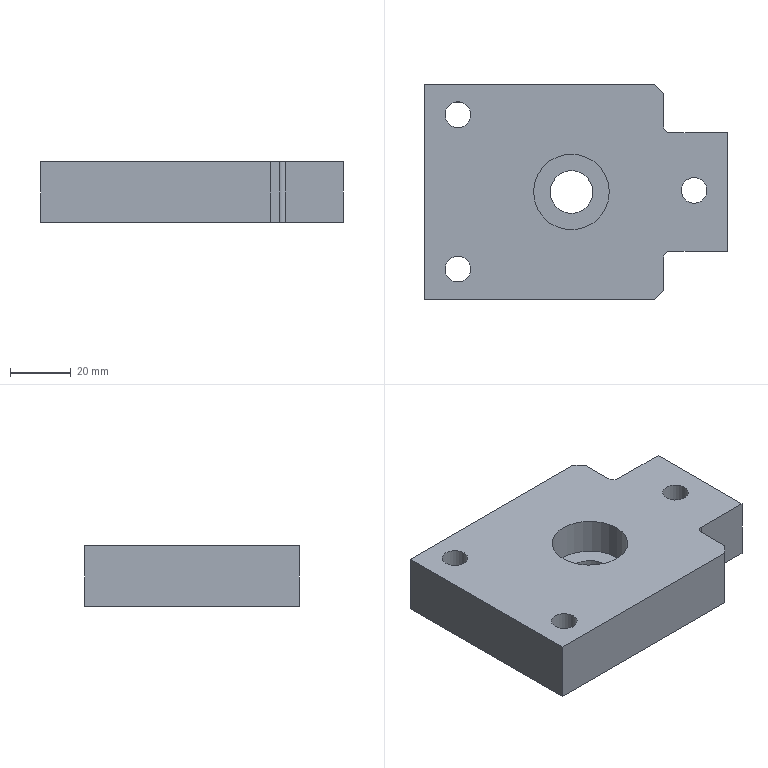Part | NX | features solid 2 | 1 solid | 26 faces | box 100 x 71 x 20 mm | volume 115003 mm3 | plane 16 | cylinder 10 | commonest cylinder face diameters 8.5 x3 14 x3 4 x2 14.1 x1 25 x1
STEP:
#1=CARTESIAN_POINT('',(232.75,0.5,10.));
#2=VERTEX_POINT('',#1);
#3=CARTESIAN_POINT('',(228.5,0.5,10.));
#4=DIRECTION('',(0.,0.,1.));
#5=DIRECTION('',(1.,0.,0.));
#6=AXIS2_PLACEMENT_3D('',#3,#4,#5);
#7=CIRCLE('',#6,4.25);
#8=EDGE_CURVE('',#2,#2,#7,.F.);
#9=ORIENTED_EDGE('',*,*,#8,.T.);
#10=EDGE_LOOP('',(#9));
#11=FACE_BOUND('',#10,.T.);
#12=CARTESIAN_POINT('',(232.75,0.5,20.));
#13=VERTEX_POINT('',#12);
#14=CARTESIAN_POINT('',(228.5,0.5,20.));
#15=DIRECTION('',(0.,0.,1.));
#16=DIRECTION('',(1.,0.,0.));
#17=AXIS2_PLACEMENT_3D('',#14,#15,#16);
#18=CIRCLE('',#17,4.25);
#19=EDGE_CURVE('',#13,#13,#18,.T.);
#20=ORIENTED_EDGE('',*,*,#19,.T.);
#21=EDGE_LOOP('',(#20));
#22=FACE_BOUND('',#21,.T.);
#23=CARTESIAN_POINT('',(228.5,0.5,40.));
#24=DIRECTION('',(0.,0.,1.));
#25=DIRECTION('',(1.,0.,0.));
#26=AXIS2_PLACEMENT_3D('',#23,#24,#25);
#27=CYLINDRICAL_SURFACE('',#26,4.25);
#28=ADVANCED_FACE('',(#11,#22),#27,.F.);
#29=ORIENTED_EDGE('',*,*,#8,.F.);
#30=EDGE_LOOP('',(#29));
#31=FACE_BOUND('',#30,.T.);
#32=CARTESIAN_POINT('',(235.5,0.5,10.));
#33=VERTEX_POINT('',#32);
#34=CARTESIAN_POINT('',(228.5,0.5,10.));
#35=DIRECTION('',(0.,0.,1.));
#36=DIRECTION('',(1.,0.,0.));
#37=AXIS2_PLACEMENT_3D('',#34,#35,#36);
#38=CIRCLE('',#37,7.);
#39=EDGE_CURVE('',#33,#33,#38,.F.);
#40=ORIENTED_EDGE('',*,*,#39,.T.);
#41=EDGE_LOOP('',(#40));
#42=FACE_BOUND('',#41,.T.);
#43=CARTESIAN_POINT('',(231.693,-4.466,10.));
#44=DIRECTION('',(0.,0.,1.));
#45=DIRECTION('',(1.,0.,0.));
#46=AXIS2_PLACEMENT_3D('',#43,#44,#45);
#47=PLANE('',#46);
#48=ADVANCED_FACE('',(#31,#42),#47,.F.);
#49=ORIENTED_EDGE('',*,*,#39,.F.);
#50=EDGE_LOOP('',(#49));
#51=FACE_BOUND('',#50,.T.);
#52=CARTESIAN_POINT('',(235.5,0.5,0.00000121));
#53=VERTEX_POINT('',#52);
#54=CARTESIAN_POINT('',(228.5,0.5,0.00000121));
#55=DIRECTION('',(0.,0.,1.));
#56=DIRECTION('',(1.,0.,0.));
#57=AXIS2_PLACEMENT_3D('',#54,#55,#56);
#58=CIRCLE('',#57,7.);
#59=EDGE_CURVE('',#53,#53,#58,.F.);
#60=ORIENTED_EDGE('',*,*,#59,.T.);
#61=EDGE_LOOP('',(#60));
#62=FACE_BOUND('',#61,.T.);
#63=CARTESIAN_POINT('',(228.5,0.5,0.00000121));
#64=DIRECTION('',(0.,0.,1.));
#65=DIRECTION('',(1.,0.,0.));
#66=AXIS2_PLACEMENT_3D('',#63,#64,#65);
#67=CYLINDRICAL_SURFACE('',#66,7.);
#68=ADVANCED_FACE('',(#51,#62),#67,.F.);
#69=CARTESIAN_POINT('',(154.75,-25.5,10.));
#70=VERTEX_POINT('',#69);
#71=CARTESIAN_POINT('',(150.5,-25.5,10.));
#72=DIRECTION('',(0.,0.,1.));
#73=DIRECTION('',(1.,0.,0.));
#74=AXIS2_PLACEMENT_3D('',#71,#72,#73);
#75=CIRCLE('',#74,4.25);
#76=EDGE_CURVE('',#70,#70,#75,.F.);
#77=ORIENTED_EDGE('',*,*,#76,.F.);
#78=EDGE_LOOP('',(#77));
#79=FACE_BOUND('',#78,.T.);
#80=CARTESIAN_POINT('',(157.5,-25.5,10.));
#81=VERTEX_POINT('',#80);
#82=CARTESIAN_POINT('',(150.5,-25.5,10.));
#83=DIRECTION('',(0.,0.,1.));
#84=DIRECTION('',(1.,0.,0.));
#85=AXIS2_PLACEMENT_3D('',#82,#83,#84);
#86=CIRCLE('',#85,7.);
#87=EDGE_CURVE('',#81,#81,#86,.F.);
#88=ORIENTED_EDGE('',*,*,#87,.T.);
#89=EDGE_LOOP('',(#88));
#90=FACE_BOUND('',#89,.T.);
#91=CARTESIAN_POINT('',(151.774,-24.174,10.));
#92=DIRECTION('',(0.,0.,1.));
#93=DIRECTION('',(1.,0.,0.));
#94=AXIS2_PLACEMENT_3D('',#91,#92,#93);
#95=PLANE('',#94);
#96=ADVANCED_FACE('',(#79,#90),#95,.F.);
#97=CARTESIAN_POINT('',(154.75,25.5,10.));
#98=VERTEX_POINT('',#97);
#99=CARTESIAN_POINT('',(150.5,25.5,10.));
#100=DIRECTION('',(0.,0.,-1.));
#101=DIRECTION('',(1.,0.,0.));
#102=AXIS2_PLACEMENT_3D('',#99,#100,#101);
#103=CIRCLE('',#102,4.25);
#104=EDGE_CURVE('',#98,#98,#103,.T.);
#105=ORIENTED_EDGE('',*,*,#104,.F.);
#106=EDGE_LOOP('',(#105));
#107=FACE_BOUND('',#106,.T.);
#108=CARTESIAN_POINT('',(157.5,25.5,10.));
#109=VERTEX_POINT('',#108);
#110=CARTESIAN_POINT('',(150.5,25.5,10.));
#111=DIRECTION('',(0.,0.,-1.));
#112=DIRECTION('',(1.,0.,0.));
#113=AXIS2_PLACEMENT_3D('',#110,#111,#112);
#114=CIRCLE('',#113,7.);
#115=EDGE_CURVE('',#109,#109,#114,.T.);
#116=ORIENTED_EDGE('',*,*,#115,.T.);
#117=EDGE_LOOP('',(#116));
#118=FACE_BOUND('',#117,.T.);
#119=CARTESIAN_POINT('',(151.774,24.174,10.));
#120=DIRECTION('',(0.,0.,1.));
#121=DIRECTION('',(1.,0.,0.));
#122=AXIS2_PLACEMENT_3D('',#119,#120,#121);
#123=PLANE('',#122);
#124=ADVANCED_FACE('',(#107,#118),#123,.F.);
#125=CARTESIAN_POINT('',(139.5,35.5,0.00000121));
#126=VERTEX_POINT('',#125);
#127=CARTESIAN_POINT('',(139.5,35.5,20.));
#128=VERTEX_POINT('',#127);
#129=CARTESIAN_POINT('',(139.5,35.5,70.));
#130=DIRECTION('',(0.,0.,1.));
#131=VECTOR('',#130,1000.);
#132=LINE('',#129,#131);
#133=EDGE_CURVE('',#126,#128,#132,.T.);
#134=ORIENTED_EDGE('',*,*,#133,.F.);
#135=CARTESIAN_POINT('',(139.5,-35.5,0.00000121));
#136=VERTEX_POINT('',#135);
#137=CARTESIAN_POINT('',(139.5,0.,0.00000121));
#138=DIRECTION('',(0.,1.,0.));
#139=VECTOR('',#138,1000.);
#140=LINE('',#137,#139);
#141=EDGE_CURVE('',#126,#136,#140,.F.);
#142=ORIENTED_EDGE('',*,*,#141,.T.);
#143=CARTESIAN_POINT('',(139.5,-35.5,20.));
#144=VERTEX_POINT('',#143);
#145=CARTESIAN_POINT('',(139.5,-35.5,70.));
#146=DIRECTION('',(0.,0.,-1.));
#147=VECTOR('',#146,1000.);
#148=LINE('',#145,#147);
#149=EDGE_CURVE('',#144,#136,#148,.T.);
#150=ORIENTED_EDGE('',*,*,#149,.F.);
#151=CARTESIAN_POINT('',(139.5,0.,20.));
#152=DIRECTION('',(0.,-1.,0.));
#153=VECTOR('',#152,1000.);
#154=LINE('',#151,#153);
#155=EDGE_CURVE('',#128,#144,#154,.T.);
#156=ORIENTED_EDGE('',*,*,#155,.F.);
#157=EDGE_LOOP('',(#134,#142,#150,#156));
#158=FACE_BOUND('',#157,.T.);
#159=CARTESIAN_POINT('',(139.5,0.,35.));
#160=DIRECTION('',(1.,0.,0.));
#161=DIRECTION('',(0.,-1.,0.));
#162=AXIS2_PLACEMENT_3D('',#159,#160,#161);
#163=PLANE('',#162);
#164=ADVANCED_FACE('',(#158),#163,.F.);
#165=ORIENTED_EDGE('',*,*,#149,.T.);
#166=CARTESIAN_POINT('',(215.5,-35.5,0.00000121));
#167=VERTEX_POINT('',#166);
#168=CARTESIAN_POINT('',(157.5,-35.5,0.00000121));
#169=DIRECTION('',(-1.,0.,0.));
#170=VECTOR('',#169,1000.);
#171=LINE('',#168,#170);
#172=EDGE_CURVE('',#136,#167,#171,.F.);
#173=ORIENTED_EDGE('',*,*,#172,.T.);
#174=CARTESIAN_POINT('',(215.5,-35.5,20.));
#175=VERTEX_POINT('',#174);
#176=CARTESIAN_POINT('',(215.5,-35.5,70.));
#177=DIRECTION('',(0.,0.,1.));
#178=VECTOR('',#177,1000.);
#179=LINE('',#176,#178);
#180=EDGE_CURVE('',#167,#175,#179,.T.);
#181=ORIENTED_EDGE('',*,*,#180,.T.);
#182=CARTESIAN_POINT('',(157.5,-35.5,20.));
#183=DIRECTION('',(1.,0.,0.));
#184=VECTOR('',#183,1000.);
#185=LINE('',#182,#184);
#186=EDGE_CURVE('',#144,#175,#185,.T.);
#187=ORIENTED_EDGE('',*,*,#186,.F.);
#188=EDGE_LOOP('',(#165,#173,#181,#187));
#189=FACE_BOUND('',#188,.T.);
#190=CARTESIAN_POINT('',(157.5,-35.5,70.));
#191=DIRECTION('',(0.,1.,0.));
#192=DIRECTION('',(-1.,0.,0.));
#193=AXIS2_PLACEMENT_3D('',#190,#191,#192);
#194=PLANE('',#193);
#195=ADVANCED_FACE('',(#189),#194,.F.);
#196=ORIENTED_EDGE('',*,*,#180,.F.);
#197=CARTESIAN_POINT('',(218.5,-32.5,0.00000121));
#198=VERTEX_POINT('',#197);
#199=CARTESIAN_POINT('',(219.5,-31.5,0.00000121));
#200=DIRECTION('',(0.7071,0.7071,0.));
#201=VECTOR('',#200,1000.);
#202=LINE('',#199,#201);
#203=EDGE_CURVE('',#198,#167,#202,.F.);
#204=ORIENTED_EDGE('',*,*,#203,.F.);
#205=CARTESIAN_POINT('',(218.5,-32.5,20.));
#206=VERTEX_POINT('',#205);
#207=CARTESIAN_POINT('',(218.5,-32.5,70.));
#208=DIRECTION('',(0.,0.,1.));
#209=VECTOR('',#208,1000.);
#210=LINE('',#207,#209);
#211=EDGE_CURVE('',#206,#198,#210,.F.);
#212=ORIENTED_EDGE('',*,*,#211,.F.);
#213=CARTESIAN_POINT('',(218.5,-32.5,20.));
#214=DIRECTION('',(0.7071,0.7071,0.));
#215=VECTOR('',#214,1000.);
#216=LINE('',#213,#215);
#217=EDGE_CURVE('',#175,#206,#216,.T.);
#218=ORIENTED_EDGE('',*,*,#217,.F.);
#219=EDGE_LOOP('',(#196,#204,#212,#218));
#220=FACE_BOUND('',#219,.T.);
#221=CARTESIAN_POINT('',(218.5,-32.5,70.));
#222=DIRECTION('',(-0.7071,0.7071,0.));
#223=DIRECTION('',(-0.7071,-0.7071,0.));
#224=AXIS2_PLACEMENT_3D('',#221,#222,#223);
#225=PLANE('',#224);
#226=ADVANCED_FACE('',(#220),#225,.F.);
#227=ORIENTED_EDGE('',*,*,#211,.T.);
#228=CARTESIAN_POINT('',(218.5,-21.558,0.00000121));
#229=VERTEX_POINT('',#228);
#230=CARTESIAN_POINT('',(218.5,0.,0.00000121));
#231=DIRECTION('',(0.,-1.,0.));
#232=VECTOR('',#231,1000.);
#233=LINE('',#230,#232);
#234=EDGE_CURVE('',#198,#229,#233,.F.);
#235=ORIENTED_EDGE('',*,*,#234,.T.);
#236=CARTESIAN_POINT('',(218.5,-21.558,20.));
#237=VERTEX_POINT('',#236);
#238=CARTESIAN_POINT('',(218.5,-21.558,20.));
#239=DIRECTION('',(0.,0.,1.));
#240=VECTOR('',#239,1000.);
#241=LINE('',#238,#240);
#242=EDGE_CURVE('',#229,#237,#241,.T.);
#243=ORIENTED_EDGE('',*,*,#242,.T.);
#244=CARTESIAN_POINT('',(218.5,-25.984,20.));
#245=DIRECTION('',(0.,-1.,0.));
#246=VECTOR('',#245,1000.);
#247=LINE('',#244,#246);
#248=EDGE_CURVE('',#206,#237,#247,.F.);
#249=ORIENTED_EDGE('',*,*,#248,.F.);
#250=EDGE_LOOP('',(#227,#235,#243,#249));
#251=FACE_BOUND('',#250,.T.);
#252=CARTESIAN_POINT('',(218.5,-33.5,70.));
#253=DIRECTION('',(-1.,0.,0.));
#254=DIRECTION('',(0.,0.,1.));
#255=AXIS2_PLACEMENT_3D('',#252,#253,#254);
#256=PLANE('',#255);
#257=ADVANCED_FACE('',(#251),#256,.F.);
#258=CARTESIAN_POINT('',(220.5,-19.558,20.));
#259=VERTEX_POINT('',#258);
#260=CARTESIAN_POINT('',(220.5,-19.558,0.00000121));
#261=VERTEX_POINT('',#260);
#262=CARTESIAN_POINT('',(220.5,-19.558,0.00000121));
#263=DIRECTION('',(0.,0.,1.));
#264=VECTOR('',#263,1000.);
#265=LINE('',#262,#264);
#266=EDGE_CURVE('',#259,#261,#265,.F.);
#267=ORIENTED_EDGE('',*,*,#266,.T.);
#268=CARTESIAN_POINT('',(239.5,-19.558,0.00000121));
#269=VERTEX_POINT('',#268);
#270=CARTESIAN_POINT('',(268.879,-19.558,0.00000121));
#271=DIRECTION('',(-1.,0.,0.));
#272=VECTOR('',#271,1000.);
#273=LINE('',#270,#272);
#274=EDGE_CURVE('',#261,#269,#273,.F.);
#275=ORIENTED_EDGE('',*,*,#274,.T.);
#276=CARTESIAN_POINT('',(239.5,-19.558,20.));
#277=VERTEX_POINT('',#276);
#278=CARTESIAN_POINT('',(239.5,-19.558,35.));
#279=DIRECTION('',(0.,0.,-1.));
#280=VECTOR('',#279,1000.);
#281=LINE('',#278,#280);
#282=EDGE_CURVE('',#269,#277,#281,.F.);
#283=ORIENTED_EDGE('',*,*,#282,.T.);
#284=CARTESIAN_POINT('',(251.29,-19.558,20.));
#285=DIRECTION('',(-1.,0.,0.));
#286=VECTOR('',#285,1000.);
#287=LINE('',#284,#286);
#288=EDGE_CURVE('',#277,#259,#287,.T.);
#289=ORIENTED_EDGE('',*,*,#288,.T.);
#290=EDGE_LOOP('',(#267,#275,#283,#289));
#291=FACE_BOUND('',#290,.T.);
#292=CARTESIAN_POINT('',(251.29,-19.558,5.));
#293=DIRECTION('',(0.,1.,0.));
#294=DIRECTION('',(0.,0.,1.));
#295=AXIS2_PLACEMENT_3D('',#292,#293,#294);
#296=PLANE('',#295);
#297=ADVANCED_FACE('',(#291),#296,.F.);
#298=ORIENTED_EDGE('',*,*,#282,.F.);
#299=CARTESIAN_POINT('',(239.5,19.558,0.00000121));
#300=VERTEX_POINT('',#299);
#301=CARTESIAN_POINT('',(239.5,0.,0.00000121));
#302=DIRECTION('',(0.,-1.,0.));
#303=VECTOR('',#302,1000.);
#304=LINE('',#301,#303);
#305=EDGE_CURVE('',#269,#300,#304,.F.);
#306=ORIENTED_EDGE('',*,*,#305,.T.);
#307=CARTESIAN_POINT('',(239.5,19.558,20.));
#308=VERTEX_POINT('',#307);
#309=CARTESIAN_POINT('',(239.5,19.558,35.));
#310=DIRECTION('',(0.,0.,1.));
#311=VECTOR('',#310,1000.);
#312=LINE('',#309,#311);
#313=EDGE_CURVE('',#308,#300,#312,.F.);
#314=ORIENTED_EDGE('',*,*,#313,.F.);
#315=CARTESIAN_POINT('',(239.5,0.,20.));
#316=DIRECTION('',(0.,1.,0.));
#317=VECTOR('',#316,1000.);
#318=LINE('',#315,#317);
#319=EDGE_CURVE('',#277,#308,#318,.T.);
#320=ORIENTED_EDGE('',*,*,#319,.F.);
#321=EDGE_LOOP('',(#298,#306,#314,#320));
#322=FACE_BOUND('',#321,.T.);
#323=CARTESIAN_POINT('',(239.5,0.,35.));
#324=DIRECTION('',(-1.,0.,0.));
#325=DIRECTION('',(0.,1.,0.));
#326=AXIS2_PLACEMENT_3D('',#323,#324,#325);
#327=PLANE('',#326);
#328=ADVANCED_FACE('',(#322),#327,.F.);
#329=ORIENTED_EDGE('',*,*,#313,.T.);
#330=CARTESIAN_POINT('',(220.5,19.558,0.00000121));
#331=VERTEX_POINT('',#330);
#332=CARTESIAN_POINT('',(268.879,19.558,0.00000121));
#333=DIRECTION('',(-1.,0.,0.));
#334=VECTOR('',#333,1000.);
#335=LINE('',#332,#334);
#336=EDGE_CURVE('',#331,#300,#335,.F.);
#337=ORIENTED_EDGE('',*,*,#336,.F.);
#338=CARTESIAN_POINT('',(220.5,19.558,20.));
#339=VERTEX_POINT('',#338);
#340=CARTESIAN_POINT('',(220.5,19.558,20.));
#341=DIRECTION('',(0.,0.,1.));
#342=VECTOR('',#341,1000.);
#343=LINE('',#340,#342);
#344=EDGE_CURVE('',#331,#339,#343,.T.);
#345=ORIENTED_EDGE('',*,*,#344,.T.);
#346=CARTESIAN_POINT('',(251.29,19.558,20.));
#347=DIRECTION('',(-1.,0.,0.));
#348=VECTOR('',#347,1000.);
#349=LINE('',#346,#348);
#350=EDGE_CURVE('',#308,#339,#349,.T.);
#351=ORIENTED_EDGE('',*,*,#350,.F.);
#352=EDGE_LOOP('',(#329,#337,#345,#351));
#353=FACE_BOUND('',#352,.T.);
#354=CARTESIAN_POINT('',(251.29,19.558,5.));
#355=DIRECTION('',(0.,-1.,0.));
#356=DIRECTION('',(0.,0.,1.));
#357=AXIS2_PLACEMENT_3D('',#354,#355,#356);
#358=PLANE('',#357);
#359=ADVANCED_FACE('',(#353),#358,.F.);
#360=CARTESIAN_POINT('',(218.5,21.558,20.));
#361=VERTEX_POINT('',#360);
#362=CARTESIAN_POINT('',(218.5,21.558,0.00000121));
#363=VERTEX_POINT('',#362);
#364=CARTESIAN_POINT('',(218.5,21.558,0.00000121));
#365=DIRECTION('',(0.,0.,1.));
#366=VECTOR('',#365,1000.);
#367=LINE('',#364,#366);
#368=EDGE_CURVE('',#361,#363,#367,.F.);
#369=ORIENTED_EDGE('',*,*,#368,.T.);
#370=CARTESIAN_POINT('',(218.5,32.5,0.00000121));
#371=VERTEX_POINT('',#370);
#372=CARTESIAN_POINT('',(218.5,0.,0.00000121));
#373=DIRECTION('',(0.,-1.,0.));
#374=VECTOR('',#373,1000.);
#375=LINE('',#372,#374);
#376=EDGE_CURVE('',#371,#363,#375,.T.);
#377=ORIENTED_EDGE('',*,*,#376,.F.);
#378=CARTESIAN_POINT('',(218.5,32.5,20.));
#379=VERTEX_POINT('',#378);
#380=CARTESIAN_POINT('',(218.5,32.5,70.));
#381=DIRECTION('',(0.,0.,-1.));
#382=VECTOR('',#381,1000.);
#383=LINE('',#380,#382);
#384=EDGE_CURVE('',#371,#379,#383,.F.);
#385=ORIENTED_EDGE('',*,*,#384,.T.);
#386=CARTESIAN_POINT('',(218.5,25.984,20.));
#387=DIRECTION('',(0.,-1.,0.));
#388=VECTOR('',#387,1000.);
#389=LINE('',#386,#388);
#390=EDGE_CURVE('',#379,#361,#389,.T.);
#391=ORIENTED_EDGE('',*,*,#390,.T.);
#392=EDGE_LOOP('',(#369,#377,#385,#391));
#393=FACE_BOUND('',#392,.T.);
#394=CARTESIAN_POINT('',(218.5,-33.5,70.));
#395=DIRECTION('',(-1.,0.,0.));
#396=DIRECTION('',(0.,0.,1.));
#397=AXIS2_PLACEMENT_3D('',#394,#395,#396);
#398=PLANE('',#397);
#399=ADVANCED_FACE('',(#393),#398,.F.);
#400=ORIENTED_EDGE('',*,*,#384,.F.);
#401=CARTESIAN_POINT('',(215.5,35.5,0.00000121));
#402=VERTEX_POINT('',#401);
#403=CARTESIAN_POINT('',(219.5,31.5,0.00000121));
#404=DIRECTION('',(-0.7071,0.7071,0.));
#405=VECTOR('',#404,1000.);
#406=LINE('',#403,#405);
#407=EDGE_CURVE('',#402,#371,#406,.F.);
#408=ORIENTED_EDGE('',*,*,#407,.F.);
#409=CARTESIAN_POINT('',(215.5,35.5,20.));
#410=VERTEX_POINT('',#409);
#411=CARTESIAN_POINT('',(215.5,35.5,70.));
#412=DIRECTION('',(0.,0.,-1.));
#413=VECTOR('',#412,1000.);
#414=LINE('',#411,#413);
#415=EDGE_CURVE('',#410,#402,#414,.T.);
#416=ORIENTED_EDGE('',*,*,#415,.F.);
#417=CARTESIAN_POINT('',(215.5,35.5,20.));
#418=DIRECTION('',(-0.7071,0.7071,0.));
#419=VECTOR('',#418,1000.);
#420=LINE('',#417,#419);
#421=EDGE_CURVE('',#379,#410,#420,.T.);
#422=ORIENTED_EDGE('',*,*,#421,.F.);
#423=EDGE_LOOP('',(#400,#408,#416,#422));
#424=FACE_BOUND('',#423,.T.);
#425=CARTESIAN_POINT('',(215.5,35.5,70.));
#426=DIRECTION('',(-0.7071,-0.7071,0.));
#427=DIRECTION('',(0.7071,-0.7071,0.));
#428=AXIS2_PLACEMENT_3D('',#425,#426,#427);
#429=PLANE('',#428);
#430=ADVANCED_FACE('',(#424),#429,.F.);
#431=ORIENTED_EDGE('',*,*,#415,.T.);
#432=CARTESIAN_POINT('',(218.5,35.5,0.00000121));
#433=DIRECTION('',(1.,0.,0.));
#434=VECTOR('',#433,1000.);
#435=LINE('',#432,#434);
#436=EDGE_CURVE('',#402,#126,#435,.F.);
#437=ORIENTED_EDGE('',*,*,#436,.T.);
#438=ORIENTED_EDGE('',*,*,#133,.T.);
#439=CARTESIAN_POINT('',(218.5,35.5,20.));
#440=DIRECTION('',(-1.,0.,0.));
#441=VECTOR('',#440,1000.);
#442=LINE('',#439,#441);
#443=EDGE_CURVE('',#410,#128,#442,.T.);
#444=ORIENTED_EDGE('',*,*,#443,.F.);
#445=EDGE_LOOP('',(#431,#437,#438,#444));
#446=FACE_BOUND('',#445,.T.);
#447=CARTESIAN_POINT('',(218.5,35.5,70.));
#448=DIRECTION('',(0.,-1.,0.));
#449=DIRECTION('',(1.,0.,0.));
#450=AXIS2_PLACEMENT_3D('',#447,#448,#449);
#451=PLANE('',#450);
#452=ADVANCED_FACE('',(#446),#451,.F.);
#453=CARTESIAN_POINT('',(200.5,0.,8.));
#454=VERTEX_POINT('',#453);
#455=CARTESIAN_POINT('',(188.,0.,8.));
#456=DIRECTION('',(0.,0.,1.));
#457=DIRECTION('',(1.,0.,0.));
#458=AXIS2_PLACEMENT_3D('',#455,#456,#457);
#459=CIRCLE('',#458,12.5);
#460=EDGE_CURVE('',#454,#454,#459,.T.);
#461=ORIENTED_EDGE('',*,*,#460,.F.);
#462=EDGE_LOOP('',(#461));
#463=FACE_BOUND('',#462,.T.);
#464=CARTESIAN_POINT('',(200.5,0.,20.));
#465=VERTEX_POINT('',#464);
#466=CARTESIAN_POINT('',(188.,0.,20.));
#467=DIRECTION('',(0.,0.,1.));
#468=DIRECTION('',(1.,0.,0.));
#469=AXIS2_PLACEMENT_3D('',#466,#467,#468);
#470=CIRCLE('',#469,12.5);
#471=EDGE_CURVE('',#465,#465,#470,.F.);
#472=ORIENTED_EDGE('',*,*,#471,.F.);
#473=EDGE_LOOP('',(#472));
#474=FACE_BOUND('',#473,.T.);
#475=CARTESIAN_POINT('',(188.,0.,2.5));
#476=DIRECTION('',(0.,0.,-1.));
#477=DIRECTION('',(-1.,0.,0.));
#478=AXIS2_PLACEMENT_3D('',#475,#476,#477);
#479=CYLINDRICAL_SURFACE('',#478,12.5);
#480=ADVANCED_FACE('',(#463,#474),#479,.F.);
#481=ORIENTED_EDGE('',*,*,#87,.F.);
#482=EDGE_LOOP('',(#481));
#483=FACE_BOUND('',#482,.T.);
#484=CARTESIAN_POINT('',(157.5,-25.5,0.00000121));
#485=VERTEX_POINT('',#484);
#486=CARTESIAN_POINT('',(150.5,-25.5,0.00000121));
#487=DIRECTION('',(0.,0.,1.));
#488=DIRECTION('',(1.,0.,0.));
#489=AXIS2_PLACEMENT_3D('',#486,#487,#488);
#490=CIRCLE('',#489,7.);
#491=EDGE_CURVE('',#485,#485,#490,.T.);
#492=ORIENTED_EDGE('',*,*,#491,.F.);
#493=EDGE_LOOP('',(#492));
#494=FACE_BOUND('',#493,.T.);
#495=CARTESIAN_POINT('',(150.5,-25.5,0.00000121));
#496=DIRECTION('',(0.,0.,1.));
#497=DIRECTION('',(1.,0.,0.));
#498=AXIS2_PLACEMENT_3D('',#495,#496,#497);
#499=CYLINDRICAL_SURFACE('',#498,7.);
#500=ADVANCED_FACE('',(#483,#494),#499,.F.);
#501=ORIENTED_EDGE('',*,*,#115,.F.);
#502=EDGE_LOOP('',(#501));
#503=FACE_BOUND('',#502,.T.);
#504=CARTESIAN_POINT('',(157.5,25.5,0.00000121));
#505=VERTEX_POINT('',#504);
#506=CARTESIAN_POINT('',(150.5,25.5,0.00000121));
#507=DIRECTION('',(0.,0.,-1.));
#508=DIRECTION('',(1.,0.,0.));
#509=AXIS2_PLACEMENT_3D('',#506,#507,#508);
#510=CIRCLE('',#509,7.);
#511=EDGE_CURVE('',#505,#505,#510,.F.);
#512=ORIENTED_EDGE('',*,*,#511,.F.);
#513=EDGE_LOOP('',(#512));
#514=FACE_BOUND('',#513,.T.);
#515=CARTESIAN_POINT('',(150.5,25.5,0.00000121));
#516=DIRECTION('',(0.,0.,1.));
#517=DIRECTION('',(1.,0.,0.));
#518=AXIS2_PLACEMENT_3D('',#515,#516,#517);
#519=CYLINDRICAL_SURFACE('',#518,7.);
#520=ADVANCED_FACE('',(#503,#514),#519,.F.);
#521=ORIENTED_EDGE('',*,*,#76,.T.);
#522=EDGE_LOOP('',(#521));
#523=FACE_BOUND('',#522,.T.);
#524=CARTESIAN_POINT('',(154.75,-25.5,20.));
#525=VERTEX_POINT('',#524);
#526=CARTESIAN_POINT('',(150.5,-25.5,20.));
#527=DIRECTION('',(0.,0.,1.));
#528=DIRECTION('',(1.,0.,0.));
#529=AXIS2_PLACEMENT_3D('',#526,#527,#528);
#530=CIRCLE('',#529,4.25);
#531=EDGE_CURVE('',#525,#525,#530,.F.);
#532=ORIENTED_EDGE('',*,*,#531,.F.);
#533=EDGE_LOOP('',(#532));
#534=FACE_BOUND('',#533,.T.);
#535=CARTESIAN_POINT('',(150.5,-25.5,40.));
#536=DIRECTION('',(0.,0.,1.));
#537=DIRECTION('',(1.,0.,0.));
#538=AXIS2_PLACEMENT_3D('',#535,#536,#537);
#539=CYLINDRICAL_SURFACE('',#538,4.25);
#540=ADVANCED_FACE('',(#523,#534),#539,.F.);
#541=ORIENTED_EDGE('',*,*,#104,.T.);
#542=EDGE_LOOP('',(#541));
#543=FACE_BOUND('',#542,.T.);
#544=CARTESIAN_POINT('',(154.75,25.5,20.));
#545=VERTEX_POINT('',#544);
#546=CARTESIAN_POINT('',(150.5,25.5,20.));
#547=DIRECTION('',(0.,0.,-1.));
#548=DIRECTION('',(1.,0.,0.));
#549=AXIS2_PLACEMENT_3D('',#546,#547,#548);
#550=CIRCLE('',#549,4.25);
#551=EDGE_CURVE('',#545,#545,#550,.T.);
#552=ORIENTED_EDGE('',*,*,#551,.F.);
#553=EDGE_LOOP('',(#552));
#554=FACE_BOUND('',#553,.T.);
#555=CARTESIAN_POINT('',(150.5,25.5,40.));
#556=DIRECTION('',(0.,0.,1.));
#557=DIRECTION('',(1.,0.,0.));
#558=AXIS2_PLACEMENT_3D('',#555,#556,#557);
#559=CYLINDRICAL_SURFACE('',#558,4.25);
#560=ADVANCED_FACE('',(#543,#554),#559,.F.);
#561=ORIENTED_EDGE('',*,*,#19,.F.);
#562=EDGE_LOOP('',(#561));
#563=FACE_BOUND('',#562,.T.);
#564=ORIENTED_EDGE('',*,*,#551,.T.);
#565=EDGE_LOOP('',(#564));
#566=FACE_BOUND('',#565,.T.);
#567=ORIENTED_EDGE('',*,*,#531,.T.);
#568=EDGE_LOOP('',(#567));
#569=FACE_BOUND('',#568,.T.);
#570=ORIENTED_EDGE('',*,*,#390,.F.);
#571=ORIENTED_EDGE('',*,*,#421,.T.);
#572=ORIENTED_EDGE('',*,*,#443,.T.);
#573=ORIENTED_EDGE('',*,*,#155,.T.);
#574=ORIENTED_EDGE('',*,*,#186,.T.);
#575=ORIENTED_EDGE('',*,*,#217,.T.);
#576=ORIENTED_EDGE('',*,*,#248,.T.);
#577=CARTESIAN_POINT('',(220.5,-21.558,20.));
#578=DIRECTION('',(0.,0.,1.));
#579=DIRECTION('',(1.,0.,0.));
#580=AXIS2_PLACEMENT_3D('',#577,#578,#579);
#581=CIRCLE('',#580,2.);
#582=EDGE_CURVE('',#237,#259,#581,.F.);
#583=ORIENTED_EDGE('',*,*,#582,.T.);
#584=ORIENTED_EDGE('',*,*,#288,.F.);
#585=ORIENTED_EDGE('',*,*,#319,.T.);
#586=ORIENTED_EDGE('',*,*,#350,.T.);
#587=CARTESIAN_POINT('',(220.5,21.558,20.));
#588=DIRECTION('',(0.,0.,1.));
#589=DIRECTION('',(1.,0.,0.));
#590=AXIS2_PLACEMENT_3D('',#587,#588,#589);
#591=CIRCLE('',#590,2.);
#592=EDGE_CURVE('',#339,#361,#591,.F.);
#593=ORIENTED_EDGE('',*,*,#592,.T.);
#594=EDGE_LOOP('',(#570,#571,#572,#573,#574,#575,#576,#583,#584,#585,#586,#593));
#595=FACE_BOUND('',#594,.T.);
#596=ORIENTED_EDGE('',*,*,#471,.T.);
#597=EDGE_LOOP('',(#596));
#598=FACE_BOUND('',#597,.T.);
#599=CARTESIAN_POINT('',(290.29,-114.016,20.));
#600=DIRECTION('',(0.,0.,1.));
#601=DIRECTION('',(1.,0.,0.));
#602=AXIS2_PLACEMENT_3D('',#599,#600,#601);
#603=PLANE('',#602);
#604=ADVANCED_FACE('',(#563,#566,#569,#595,#598),#603,.T.);
#605=ORIENTED_EDGE('',*,*,#344,.F.);
#606=CARTESIAN_POINT('',(220.5,21.558,0.00000121));
#607=DIRECTION('',(0.,0.,-1.));
#608=DIRECTION('',(-1.,0.,0.));
#609=AXIS2_PLACEMENT_3D('',#606,#607,#608);
#610=CIRCLE('',#609,2.);
#611=EDGE_CURVE('',#363,#331,#610,.F.);
#612=ORIENTED_EDGE('',*,*,#611,.F.);
#613=ORIENTED_EDGE('',*,*,#368,.F.);
#614=ORIENTED_EDGE('',*,*,#592,.F.);
#615=EDGE_LOOP('',(#605,#612,#613,#614));
#616=FACE_BOUND('',#615,.T.);
#617=CARTESIAN_POINT('',(220.5,21.558,5.));
#618=DIRECTION('',(0.,0.,-1.));
#619=DIRECTION('',(-1.,0.,0.));
#620=AXIS2_PLACEMENT_3D('',#617,#618,#619);
#621=CYLINDRICAL_SURFACE('',#620,2.);
#622=ADVANCED_FACE('',(#616),#621,.F.);
#623=ORIENTED_EDGE('',*,*,#242,.F.);
#624=CARTESIAN_POINT('',(220.5,-21.558,0.00000121));
#625=DIRECTION('',(0.,0.,-1.));
#626=DIRECTION('',(-1.,0.,0.));
#627=AXIS2_PLACEMENT_3D('',#624,#625,#626);
#628=CIRCLE('',#627,2.);
#629=EDGE_CURVE('',#261,#229,#628,.F.);
#630=ORIENTED_EDGE('',*,*,#629,.F.);
#631=ORIENTED_EDGE('',*,*,#266,.F.);
#632=ORIENTED_EDGE('',*,*,#582,.F.);
#633=EDGE_LOOP('',(#623,#630,#631,#632));
#634=FACE_BOUND('',#633,.T.);
#635=CARTESIAN_POINT('',(220.5,-21.558,70.));
#636=DIRECTION('',(0.,0.,-1.));
#637=DIRECTION('',(-1.,0.,0.));
#638=AXIS2_PLACEMENT_3D('',#635,#636,#637);
#639=CYLINDRICAL_SURFACE('',#638,2.);
#640=ADVANCED_FACE('',(#634),#639,.F.);
#641=ORIENTED_EDGE('',*,*,#460,.T.);
#642=EDGE_LOOP('',(#641));
#643=FACE_BOUND('',#642,.T.);
#644=CARTESIAN_POINT('',(195.05,0.,8.));
#645=VERTEX_POINT('',#644);
#646=CARTESIAN_POINT('',(188.,0.,8.));
#647=DIRECTION('',(0.,0.,1.));
#648=DIRECTION('',(1.,0.,0.));
#649=AXIS2_PLACEMENT_3D('',#646,#647,#648);
#650=CIRCLE('',#649,7.05);
#651=EDGE_CURVE('',#645,#645,#650,.F.);
#652=ORIENTED_EDGE('',*,*,#651,.T.);
#653=EDGE_LOOP('',(#652));
#654=FACE_BOUND('',#653,.T.);
#655=CARTESIAN_POINT('',(189.5,0.,8.));
#656=DIRECTION('',(0.,0.,1.));
#657=DIRECTION('',(1.,0.,0.));
#658=AXIS2_PLACEMENT_3D('',#655,#656,#657);
#659=PLANE('',#658);
#660=ADVANCED_FACE('',(#643,#654),#659,.T.);
#661=CARTESIAN_POINT('',(180.95,0.,0.00000121));
#662=VERTEX_POINT('',#661);
#663=CARTESIAN_POINT('',(188.,0.,0.00000121));
#664=DIRECTION('',(0.,0.,-1.));
#665=DIRECTION('',(-1.,0.,0.));
#666=AXIS2_PLACEMENT_3D('',#663,#664,#665);
#667=CIRCLE('',#666,7.05);
#668=EDGE_CURVE('',#662,#662,#667,.F.);
#669=ORIENTED_EDGE('',*,*,#668,.F.);
#670=EDGE_LOOP('',(#669));
#671=FACE_BOUND('',#670,.T.);
#672=ORIENTED_EDGE('',*,*,#651,.F.);
#673=EDGE_LOOP('',(#672));
#674=FACE_BOUND('',#673,.T.);
#675=CARTESIAN_POINT('',(188.,0.,2.5));
#676=DIRECTION('',(0.,0.,-1.));
#677=DIRECTION('',(-1.,0.,0.));
#678=AXIS2_PLACEMENT_3D('',#675,#676,#677);
#679=CYLINDRICAL_SURFACE('',#678,7.05);
#680=ADVANCED_FACE('',(#671,#674),#679,.F.);
#681=ORIENTED_EDGE('',*,*,#59,.F.);
#682=EDGE_LOOP('',(#681));
#683=FACE_BOUND('',#682,.T.);
#684=ORIENTED_EDGE('',*,*,#511,.T.);
#685=EDGE_LOOP('',(#684));
#686=FACE_BOUND('',#685,.T.);
#687=ORIENTED_EDGE('',*,*,#491,.T.);
#688=EDGE_LOOP('',(#687));
#689=FACE_BOUND('',#688,.T.);
#690=ORIENTED_EDGE('',*,*,#668,.T.);
#691=EDGE_LOOP('',(#690));
#692=FACE_BOUND('',#691,.T.);
#693=ORIENTED_EDGE('',*,*,#436,.F.);
#694=ORIENTED_EDGE('',*,*,#407,.T.);
#695=ORIENTED_EDGE('',*,*,#376,.T.);
#696=ORIENTED_EDGE('',*,*,#611,.T.);
#697=ORIENTED_EDGE('',*,*,#336,.T.);
#698=ORIENTED_EDGE('',*,*,#305,.F.);
#699=ORIENTED_EDGE('',*,*,#274,.F.);
#700=ORIENTED_EDGE('',*,*,#629,.T.);
#701=ORIENTED_EDGE('',*,*,#234,.F.);
#702=ORIENTED_EDGE('',*,*,#203,.T.);
#703=ORIENTED_EDGE('',*,*,#172,.F.);
#704=ORIENTED_EDGE('',*,*,#141,.F.);
#705=EDGE_LOOP('',(#693,#694,#695,#696,#697,#698,#699,#700,#701,#702,#703,#704));
#706=FACE_BOUND('',#705,.T.);
#707=CARTESIAN_POINT('',(188.,0.,0.00000121));
#708=DIRECTION('',(0.,0.,-1.));
#709=DIRECTION('',(-1.,0.,0.));
#710=AXIS2_PLACEMENT_3D('',#707,#708,#709);
#711=PLANE('',#710);
#712=ADVANCED_FACE('',(#683,#686,#689,#692,#706),#711,.T.);
#713=CLOSED_SHELL('',(#28,#48,#68,#96,#124,#164,#195,#226,#257,#297,#328,#359,#399,#430,#452,#480,#500,#520,#540,#560,#604,#622,#640,#660,#680,#712));
#714=MANIFOLD_SOLID_BREP('',#713);
#715=(LENGTH_UNIT()NAMED_UNIT(*)SI_UNIT(.MILLI.,.METRE.));
#716=UNCERTAINTY_MEASURE_WITH_UNIT(LENGTH_MEASURE(0.00001),#715,'','');
#717=(NAMED_UNIT(*)PLANE_ANGLE_UNIT()SI_UNIT($,.RADIAN.));
#718=(NAMED_UNIT(*)SI_UNIT($,.STERADIAN.)SOLID_ANGLE_UNIT());
#719=(GEOMETRIC_REPRESENTATION_CONTEXT(3)GLOBAL_UNCERTAINTY_ASSIGNED_CONTEXT((#716))GLOBAL_UNIT_ASSIGNED_CONTEXT((#715,#717,#718))REPRESENTATION_CONTEXT('',''));
#720=ADVANCED_BREP_SHAPE_REPRESENTATION('',(#714),#719);